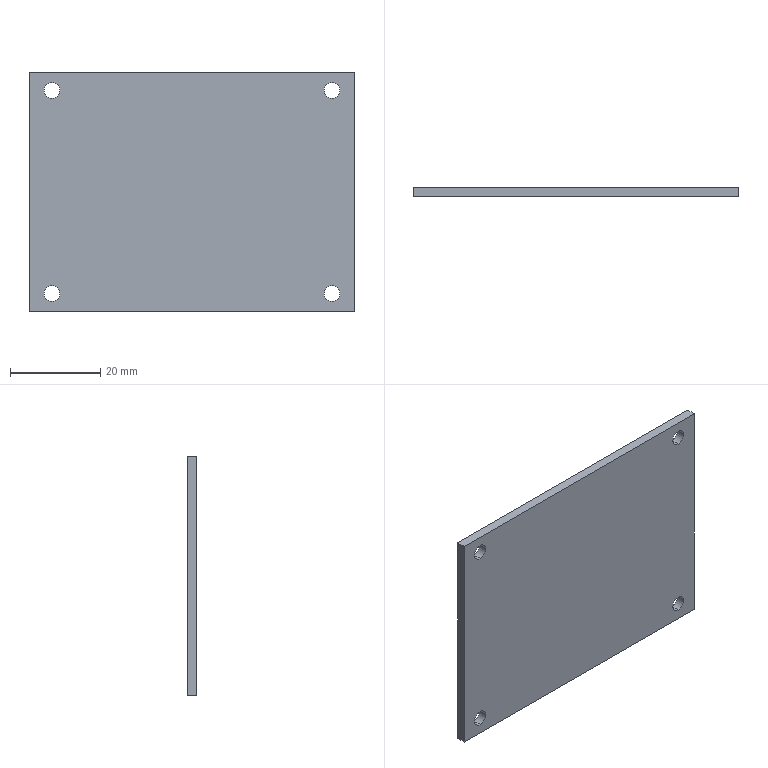Part | SolidWorks | features BaseBody 1 | 1 solid | 14 faces | box 72 x 2 x 53 mm | volume 7555 mm3 | cylinder 8 | plane 6 | commonest cylinder face diameters 3.5 x8
STEP:
#1=CARTESIAN_POINT('',(-31.,2.,24.25));
#2=VERTEX_POINT('',#1);
#3=CARTESIAN_POINT('',(-31.,0.,24.25));
#4=VERTEX_POINT('',#3);
#5=CARTESIAN_POINT('',(-31.,2.,24.25));
#6=DIRECTION('',(0.,-1.,0.));
#7=VECTOR('',#6,1000.);
#8=LINE('',#5,#7);
#9=EDGE_CURVE('',#2,#4,#8,.T.);
#10=ORIENTED_EDGE('',*,*,#9,.F.);
#11=CARTESIAN_POINT('',(-31.,2.,20.75));
#12=VERTEX_POINT('',#11);
#13=CARTESIAN_POINT('',(-31.,2.,22.5));
#14=DIRECTION('',(0.,1.,0.));
#15=DIRECTION('',(0.,0.,-1.));
#16=AXIS2_PLACEMENT_3D('',#13,#14,#15);
#17=CIRCLE('',#16,1.75);
#18=EDGE_CURVE('',#2,#12,#17,.T.);
#19=ORIENTED_EDGE('',*,*,#18,.T.);
#20=CARTESIAN_POINT('',(-31.,0.,20.75));
#21=VERTEX_POINT('',#20);
#22=CARTESIAN_POINT('',(-31.,2.,20.75));
#23=DIRECTION('',(0.,-1.,0.));
#24=VECTOR('',#23,1000.);
#25=LINE('',#22,#24);
#26=EDGE_CURVE('',#12,#21,#25,.T.);
#27=ORIENTED_EDGE('',*,*,#26,.T.);
#28=CARTESIAN_POINT('',(-31.,0.,22.5));
#29=DIRECTION('',(0.,1.,0.));
#30=DIRECTION('',(0.,0.,-1.));
#31=AXIS2_PLACEMENT_3D('',#28,#29,#30);
#32=CIRCLE('',#31,1.75);
#33=EDGE_CURVE('',#4,#21,#32,.T.);
#34=ORIENTED_EDGE('',*,*,#33,.F.);
#35=EDGE_LOOP('',(#10,#19,#27,#34));
#36=FACE_OUTER_BOUND('',#35,.T.);
#37=CARTESIAN_POINT('',(-31.,2.,22.5));
#38=DIRECTION('',(0.,-1.,0.));
#39=DIRECTION('',(0.,0.,-1.));
#40=AXIS2_PLACEMENT_3D('',#37,#38,#39);
#41=CYLINDRICAL_SURFACE('',#40,1.75);
#42=ADVANCED_FACE('',(#36),#41,.F.);
#43=CARTESIAN_POINT('',(31.,2.,24.25));
#44=VERTEX_POINT('',#43);
#45=CARTESIAN_POINT('',(31.,0.,24.25));
#46=VERTEX_POINT('',#45);
#47=CARTESIAN_POINT('',(31.,2.,24.25));
#48=DIRECTION('',(0.,-1.,0.));
#49=VECTOR('',#48,1000.);
#50=LINE('',#47,#49);
#51=EDGE_CURVE('',#44,#46,#50,.T.);
#52=ORIENTED_EDGE('',*,*,#51,.F.);
#53=CARTESIAN_POINT('',(31.,2.,20.75));
#54=VERTEX_POINT('',#53);
#55=CARTESIAN_POINT('',(31.,2.,22.5));
#56=DIRECTION('',(0.,1.,0.));
#57=DIRECTION('',(0.,0.,1.));
#58=AXIS2_PLACEMENT_3D('',#55,#56,#57);
#59=CIRCLE('',#58,1.75);
#60=EDGE_CURVE('',#44,#54,#59,.T.);
#61=ORIENTED_EDGE('',*,*,#60,.T.);
#62=CARTESIAN_POINT('',(31.,0.,20.75));
#63=VERTEX_POINT('',#62);
#64=CARTESIAN_POINT('',(31.,2.,20.75));
#65=DIRECTION('',(0.,-1.,0.));
#66=VECTOR('',#65,1000.);
#67=LINE('',#64,#66);
#68=EDGE_CURVE('',#54,#63,#67,.T.);
#69=ORIENTED_EDGE('',*,*,#68,.T.);
#70=CARTESIAN_POINT('',(31.,0.,22.5));
#71=DIRECTION('',(0.,1.,0.));
#72=DIRECTION('',(0.,0.,1.));
#73=AXIS2_PLACEMENT_3D('',#70,#71,#72);
#74=CIRCLE('',#73,1.75);
#75=EDGE_CURVE('',#46,#63,#74,.T.);
#76=ORIENTED_EDGE('',*,*,#75,.F.);
#77=EDGE_LOOP('',(#52,#61,#69,#76));
#78=FACE_OUTER_BOUND('',#77,.T.);
#79=CARTESIAN_POINT('',(31.,2.,22.5));
#80=DIRECTION('',(0.,-1.,0.));
#81=DIRECTION('',(0.,0.,-1.));
#82=AXIS2_PLACEMENT_3D('',#79,#80,#81);
#83=CYLINDRICAL_SURFACE('',#82,1.75);
#84=ADVANCED_FACE('',(#78),#83,.F.);
#85=CARTESIAN_POINT('',(31.,2.,-20.75));
#86=VERTEX_POINT('',#85);
#87=CARTESIAN_POINT('',(31.,0.,-20.75));
#88=VERTEX_POINT('',#87);
#89=CARTESIAN_POINT('',(31.,2.,-20.75));
#90=DIRECTION('',(0.,-1.,0.));
#91=VECTOR('',#90,1000.);
#92=LINE('',#89,#91);
#93=EDGE_CURVE('',#86,#88,#92,.T.);
#94=ORIENTED_EDGE('',*,*,#93,.F.);
#95=CARTESIAN_POINT('',(31.,2.,-24.25));
#96=VERTEX_POINT('',#95);
#97=CARTESIAN_POINT('',(31.,2.,-22.5));
#98=DIRECTION('',(0.,1.,0.));
#99=DIRECTION('',(0.,0.,-1.));
#100=AXIS2_PLACEMENT_3D('',#97,#98,#99);
#101=CIRCLE('',#100,1.75);
#102=EDGE_CURVE('',#86,#96,#101,.T.);
#103=ORIENTED_EDGE('',*,*,#102,.T.);
#104=CARTESIAN_POINT('',(31.,0.,-24.25));
#105=VERTEX_POINT('',#104);
#106=CARTESIAN_POINT('',(31.,2.,-24.25));
#107=DIRECTION('',(0.,-1.,0.));
#108=VECTOR('',#107,1000.);
#109=LINE('',#106,#108);
#110=EDGE_CURVE('',#96,#105,#109,.T.);
#111=ORIENTED_EDGE('',*,*,#110,.T.);
#112=CARTESIAN_POINT('',(31.,0.,-22.5));
#113=DIRECTION('',(0.,1.,0.));
#114=DIRECTION('',(0.,0.,-1.));
#115=AXIS2_PLACEMENT_3D('',#112,#113,#114);
#116=CIRCLE('',#115,1.75);
#117=EDGE_CURVE('',#88,#105,#116,.T.);
#118=ORIENTED_EDGE('',*,*,#117,.F.);
#119=EDGE_LOOP('',(#94,#103,#111,#118));
#120=FACE_OUTER_BOUND('',#119,.T.);
#121=CARTESIAN_POINT('',(31.,2.,-22.5));
#122=DIRECTION('',(0.,-1.,0.));
#123=DIRECTION('',(0.,0.,-1.));
#124=AXIS2_PLACEMENT_3D('',#121,#122,#123);
#125=CYLINDRICAL_SURFACE('',#124,1.75);
#126=ADVANCED_FACE('',(#120),#125,.F.);
#127=CARTESIAN_POINT('',(-31.,2.,-20.75));
#128=VERTEX_POINT('',#127);
#129=CARTESIAN_POINT('',(-31.,0.,-20.75));
#130=VERTEX_POINT('',#129);
#131=CARTESIAN_POINT('',(-31.,2.,-20.75));
#132=DIRECTION('',(0.,-1.,0.));
#133=VECTOR('',#132,1000.);
#134=LINE('',#131,#133);
#135=EDGE_CURVE('',#128,#130,#134,.T.);
#136=ORIENTED_EDGE('',*,*,#135,.F.);
#137=CARTESIAN_POINT('',(-31.,2.,-24.25));
#138=VERTEX_POINT('',#137);
#139=CARTESIAN_POINT('',(-31.,2.,-22.5));
#140=DIRECTION('',(0.,1.,0.));
#141=DIRECTION('',(0.,0.,1.));
#142=AXIS2_PLACEMENT_3D('',#139,#140,#141);
#143=CIRCLE('',#142,1.75);
#144=EDGE_CURVE('',#128,#138,#143,.T.);
#145=ORIENTED_EDGE('',*,*,#144,.T.);
#146=CARTESIAN_POINT('',(-31.,0.,-24.25));
#147=VERTEX_POINT('',#146);
#148=CARTESIAN_POINT('',(-31.,2.,-24.25));
#149=DIRECTION('',(0.,-1.,0.));
#150=VECTOR('',#149,1000.);
#151=LINE('',#148,#150);
#152=EDGE_CURVE('',#138,#147,#151,.T.);
#153=ORIENTED_EDGE('',*,*,#152,.T.);
#154=CARTESIAN_POINT('',(-31.,0.,-22.5));
#155=DIRECTION('',(0.,1.,0.));
#156=DIRECTION('',(0.,0.,1.));
#157=AXIS2_PLACEMENT_3D('',#154,#155,#156);
#158=CIRCLE('',#157,1.75);
#159=EDGE_CURVE('',#130,#147,#158,.T.);
#160=ORIENTED_EDGE('',*,*,#159,.F.);
#161=EDGE_LOOP('',(#136,#145,#153,#160));
#162=FACE_OUTER_BOUND('',#161,.T.);
#163=CARTESIAN_POINT('',(-31.,2.,-22.5));
#164=DIRECTION('',(0.,-1.,0.));
#165=DIRECTION('',(0.,0.,-1.));
#166=AXIS2_PLACEMENT_3D('',#163,#164,#165);
#167=CYLINDRICAL_SURFACE('',#166,1.75);
#168=ADVANCED_FACE('',(#162),#167,.F.);
#169=CARTESIAN_POINT('',(-36.,0.,26.5));
#170=VERTEX_POINT('',#169);
#171=CARTESIAN_POINT('',(36.,0.,26.5));
#172=VERTEX_POINT('',#171);
#173=CARTESIAN_POINT('',(-36.,0.,26.5));
#174=DIRECTION('',(1.,0.,0.));
#175=VECTOR('',#174,1000.);
#176=LINE('',#173,#175);
#177=EDGE_CURVE('',#170,#172,#176,.T.);
#178=ORIENTED_EDGE('',*,*,#177,.T.);
#179=CARTESIAN_POINT('',(36.,2.,26.5));
#180=VERTEX_POINT('',#179);
#181=CARTESIAN_POINT('',(36.,2.,26.5));
#182=DIRECTION('',(0.,-1.,0.));
#183=VECTOR('',#182,1000.);
#184=LINE('',#181,#183);
#185=EDGE_CURVE('',#180,#172,#184,.T.);
#186=ORIENTED_EDGE('',*,*,#185,.F.);
#187=CARTESIAN_POINT('',(-36.,2.,26.5));
#188=VERTEX_POINT('',#187);
#189=CARTESIAN_POINT('',(-36.,2.,26.5));
#190=DIRECTION('',(1.,0.,0.));
#191=VECTOR('',#190,1000.);
#192=LINE('',#189,#191);
#193=EDGE_CURVE('',#188,#180,#192,.T.);
#194=ORIENTED_EDGE('',*,*,#193,.F.);
#195=CARTESIAN_POINT('',(-36.,2.,26.5));
#196=DIRECTION('',(0.,-1.,0.));
#197=VECTOR('',#196,1000.);
#198=LINE('',#195,#197);
#199=EDGE_CURVE('',#188,#170,#198,.T.);
#200=ORIENTED_EDGE('',*,*,#199,.T.);
#201=EDGE_LOOP('',(#178,#186,#194,#200));
#202=FACE_OUTER_BOUND('',#201,.T.);
#203=CARTESIAN_POINT('',(-36.,2.,26.5));
#204=DIRECTION('',(0.,0.,-1.));
#205=DIRECTION('',(0.,-1.,0.));
#206=AXIS2_PLACEMENT_3D('',#203,#204,#205);
#207=PLANE('',#206);
#208=ADVANCED_FACE('',(#202),#207,.F.);
#209=CARTESIAN_POINT('',(-36.,0.,-26.5));
#210=VERTEX_POINT('',#209);
#211=CARTESIAN_POINT('',(-36.,0.,-26.5));
#212=DIRECTION('',(0.,0.,1.));
#213=VECTOR('',#212,1000.);
#214=LINE('',#211,#213);
#215=EDGE_CURVE('',#210,#170,#214,.T.);
#216=ORIENTED_EDGE('',*,*,#215,.T.);
#217=ORIENTED_EDGE('',*,*,#199,.F.);
#218=CARTESIAN_POINT('',(-36.,2.,-26.5));
#219=VERTEX_POINT('',#218);
#220=CARTESIAN_POINT('',(-36.,2.,-26.5));
#221=DIRECTION('',(0.,0.,1.));
#222=VECTOR('',#221,1000.);
#223=LINE('',#220,#222);
#224=EDGE_CURVE('',#219,#188,#223,.T.);
#225=ORIENTED_EDGE('',*,*,#224,.F.);
#226=CARTESIAN_POINT('',(-36.,2.,-26.5));
#227=DIRECTION('',(0.,-1.,0.));
#228=VECTOR('',#227,1000.);
#229=LINE('',#226,#228);
#230=EDGE_CURVE('',#219,#210,#229,.T.);
#231=ORIENTED_EDGE('',*,*,#230,.T.);
#232=EDGE_LOOP('',(#216,#217,#225,#231));
#233=FACE_OUTER_BOUND('',#232,.T.);
#234=CARTESIAN_POINT('',(-36.,2.,-26.5));
#235=DIRECTION('',(1.,0.,0.));
#236=DIRECTION('',(0.,1.,0.));
#237=AXIS2_PLACEMENT_3D('',#234,#235,#236);
#238=PLANE('',#237);
#239=ADVANCED_FACE('',(#233),#238,.F.);
#240=CARTESIAN_POINT('',(36.,0.,-26.5));
#241=VERTEX_POINT('',#240);
#242=CARTESIAN_POINT('',(-36.,0.,-26.5));
#243=DIRECTION('',(-1.,0.,0.));
#244=VECTOR('',#243,1000.);
#245=LINE('',#242,#244);
#246=EDGE_CURVE('',#241,#210,#245,.T.);
#247=ORIENTED_EDGE('',*,*,#246,.T.);
#248=ORIENTED_EDGE('',*,*,#230,.F.);
#249=CARTESIAN_POINT('',(36.,2.,-26.5));
#250=VERTEX_POINT('',#249);
#251=CARTESIAN_POINT('',(-36.,2.,-26.5));
#252=DIRECTION('',(-1.,0.,0.));
#253=VECTOR('',#252,1000.);
#254=LINE('',#251,#253);
#255=EDGE_CURVE('',#250,#219,#254,.T.);
#256=ORIENTED_EDGE('',*,*,#255,.F.);
#257=CARTESIAN_POINT('',(36.,2.,-26.5));
#258=DIRECTION('',(0.,-1.,0.));
#259=VECTOR('',#258,1000.);
#260=LINE('',#257,#259);
#261=EDGE_CURVE('',#250,#241,#260,.T.);
#262=ORIENTED_EDGE('',*,*,#261,.T.);
#263=EDGE_LOOP('',(#247,#248,#256,#262));
#264=FACE_OUTER_BOUND('',#263,.T.);
#265=CARTESIAN_POINT('',(-36.,2.,-26.5));
#266=DIRECTION('',(0.,0.,1.));
#267=DIRECTION('',(1.,0.,0.));
#268=AXIS2_PLACEMENT_3D('',#265,#266,#267);
#269=PLANE('',#268);
#270=ADVANCED_FACE('',(#264),#269,.F.);
#271=CARTESIAN_POINT('',(36.,0.,-26.5));
#272=DIRECTION('',(0.,0.,-1.));
#273=VECTOR('',#272,1000.);
#274=LINE('',#271,#273);
#275=EDGE_CURVE('',#172,#241,#274,.T.);
#276=ORIENTED_EDGE('',*,*,#275,.T.);
#277=ORIENTED_EDGE('',*,*,#261,.F.);
#278=CARTESIAN_POINT('',(36.,2.,-26.5));
#279=DIRECTION('',(0.,0.,-1.));
#280=VECTOR('',#279,1000.);
#281=LINE('',#278,#280);
#282=EDGE_CURVE('',#180,#250,#281,.T.);
#283=ORIENTED_EDGE('',*,*,#282,.F.);
#284=ORIENTED_EDGE('',*,*,#185,.T.);
#285=EDGE_LOOP('',(#276,#277,#283,#284));
#286=FACE_OUTER_BOUND('',#285,.T.);
#287=CARTESIAN_POINT('',(36.,2.,-26.5));
#288=DIRECTION('',(-1.,0.,0.));
#289=DIRECTION('',(0.,1.,0.));
#290=AXIS2_PLACEMENT_3D('',#287,#288,#289);
#291=PLANE('',#290);
#292=ADVANCED_FACE('',(#286),#291,.F.);
#293=CARTESIAN_POINT('',(-31.,0.,22.5));
#294=DIRECTION('',(0.,1.,0.));
#295=DIRECTION('',(0.,0.,-1.));
#296=AXIS2_PLACEMENT_3D('',#293,#294,#295);
#297=CIRCLE('',#296,1.75);
#298=EDGE_CURVE('',#21,#4,#297,.T.);
#299=ORIENTED_EDGE('',*,*,#298,.T.);
#300=ORIENTED_EDGE('',*,*,#33,.T.);
#301=EDGE_LOOP('',(#299,#300));
#302=FACE_BOUND('',#301,.T.);
#303=CARTESIAN_POINT('',(31.,0.,22.5));
#304=DIRECTION('',(0.,1.,0.));
#305=DIRECTION('',(0.,0.,1.));
#306=AXIS2_PLACEMENT_3D('',#303,#304,#305);
#307=CIRCLE('',#306,1.75);
#308=EDGE_CURVE('',#63,#46,#307,.T.);
#309=ORIENTED_EDGE('',*,*,#308,.T.);
#310=ORIENTED_EDGE('',*,*,#75,.T.);
#311=EDGE_LOOP('',(#309,#310));
#312=FACE_BOUND('',#311,.T.);
#313=CARTESIAN_POINT('',(31.,0.,-22.5));
#314=DIRECTION('',(0.,1.,0.));
#315=DIRECTION('',(0.,0.,-1.));
#316=AXIS2_PLACEMENT_3D('',#313,#314,#315);
#317=CIRCLE('',#316,1.75);
#318=EDGE_CURVE('',#105,#88,#317,.T.);
#319=ORIENTED_EDGE('',*,*,#318,.T.);
#320=ORIENTED_EDGE('',*,*,#117,.T.);
#321=EDGE_LOOP('',(#319,#320));
#322=FACE_BOUND('',#321,.T.);
#323=CARTESIAN_POINT('',(-31.,0.,-22.5));
#324=DIRECTION('',(0.,1.,0.));
#325=DIRECTION('',(0.,0.,1.));
#326=AXIS2_PLACEMENT_3D('',#323,#324,#325);
#327=CIRCLE('',#326,1.75);
#328=EDGE_CURVE('',#147,#130,#327,.T.);
#329=ORIENTED_EDGE('',*,*,#328,.T.);
#330=ORIENTED_EDGE('',*,*,#159,.T.);
#331=EDGE_LOOP('',(#329,#330));
#332=FACE_BOUND('',#331,.T.);
#333=ORIENTED_EDGE('',*,*,#275,.F.);
#334=ORIENTED_EDGE('',*,*,#177,.F.);
#335=ORIENTED_EDGE('',*,*,#215,.F.);
#336=ORIENTED_EDGE('',*,*,#246,.F.);
#337=EDGE_LOOP('',(#333,#334,#335,#336));
#338=FACE_OUTER_BOUND('',#337,.T.);
#339=CARTESIAN_POINT('',(0.,0.,0.));
#340=DIRECTION('',(0.,1.,0.));
#341=DIRECTION('',(1.,0.,0.));
#342=AXIS2_PLACEMENT_3D('',#339,#340,#341);
#343=PLANE('',#342);
#344=ADVANCED_FACE('',(#302,#312,#322,#332,#338),#343,.F.);
#345=CARTESIAN_POINT('',(-31.,2.,22.5));
#346=DIRECTION('',(0.,1.,0.));
#347=DIRECTION('',(0.,0.,-1.));
#348=AXIS2_PLACEMENT_3D('',#345,#346,#347);
#349=CIRCLE('',#348,1.75);
#350=EDGE_CURVE('',#12,#2,#349,.T.);
#351=ORIENTED_EDGE('',*,*,#350,.F.);
#352=ORIENTED_EDGE('',*,*,#18,.F.);
#353=EDGE_LOOP('',(#351,#352));
#354=FACE_BOUND('',#353,.T.);
#355=CARTESIAN_POINT('',(31.,2.,-22.5));
#356=DIRECTION('',(0.,1.,0.));
#357=DIRECTION('',(0.,0.,-1.));
#358=AXIS2_PLACEMENT_3D('',#355,#356,#357);
#359=CIRCLE('',#358,1.75);
#360=EDGE_CURVE('',#96,#86,#359,.T.);
#361=ORIENTED_EDGE('',*,*,#360,.F.);
#362=ORIENTED_EDGE('',*,*,#102,.F.);
#363=EDGE_LOOP('',(#361,#362));
#364=FACE_BOUND('',#363,.T.);
#365=CARTESIAN_POINT('',(-31.,2.,-22.5));
#366=DIRECTION('',(0.,1.,0.));
#367=DIRECTION('',(0.,0.,1.));
#368=AXIS2_PLACEMENT_3D('',#365,#366,#367);
#369=CIRCLE('',#368,1.75);
#370=EDGE_CURVE('',#138,#128,#369,.T.);
#371=ORIENTED_EDGE('',*,*,#370,.F.);
#372=ORIENTED_EDGE('',*,*,#144,.F.);
#373=EDGE_LOOP('',(#371,#372));
#374=FACE_BOUND('',#373,.T.);
#375=CARTESIAN_POINT('',(31.,2.,22.5));
#376=DIRECTION('',(0.,1.,0.));
#377=DIRECTION('',(0.,0.,1.));
#378=AXIS2_PLACEMENT_3D('',#375,#376,#377);
#379=CIRCLE('',#378,1.75);
#380=EDGE_CURVE('',#54,#44,#379,.T.);
#381=ORIENTED_EDGE('',*,*,#380,.F.);
#382=ORIENTED_EDGE('',*,*,#60,.F.);
#383=EDGE_LOOP('',(#381,#382));
#384=FACE_BOUND('',#383,.T.);
#385=ORIENTED_EDGE('',*,*,#282,.T.);
#386=ORIENTED_EDGE('',*,*,#255,.T.);
#387=ORIENTED_EDGE('',*,*,#224,.T.);
#388=ORIENTED_EDGE('',*,*,#193,.T.);
#389=EDGE_LOOP('',(#385,#386,#387,#388));
#390=FACE_OUTER_BOUND('',#389,.T.);
#391=CARTESIAN_POINT('',(0.,2.,0.));
#392=DIRECTION('',(0.,1.,0.));
#393=DIRECTION('',(1.,0.,0.));
#394=AXIS2_PLACEMENT_3D('',#391,#392,#393);
#395=PLANE('',#394);
#396=ADVANCED_FACE('',(#354,#364,#374,#384,#390),#395,.T.);
#397=ORIENTED_EDGE('',*,*,#370,.T.);
#398=ORIENTED_EDGE('',*,*,#135,.T.);
#399=ORIENTED_EDGE('',*,*,#328,.F.);
#400=ORIENTED_EDGE('',*,*,#152,.F.);
#401=EDGE_LOOP('',(#397,#398,#399,#400));
#402=FACE_OUTER_BOUND('',#401,.T.);
#403=CARTESIAN_POINT('',(-31.,2.,-22.5));
#404=DIRECTION('',(0.,-1.,0.));
#405=DIRECTION('',(0.,0.,-1.));
#406=AXIS2_PLACEMENT_3D('',#403,#404,#405);
#407=CYLINDRICAL_SURFACE('',#406,1.75);
#408=ADVANCED_FACE('',(#402),#407,.F.);
#409=ORIENTED_EDGE('',*,*,#360,.T.);
#410=ORIENTED_EDGE('',*,*,#93,.T.);
#411=ORIENTED_EDGE('',*,*,#318,.F.);
#412=ORIENTED_EDGE('',*,*,#110,.F.);
#413=EDGE_LOOP('',(#409,#410,#411,#412));
#414=FACE_OUTER_BOUND('',#413,.T.);
#415=CARTESIAN_POINT('',(31.,2.,-22.5));
#416=DIRECTION('',(0.,-1.,0.));
#417=DIRECTION('',(0.,0.,-1.));
#418=AXIS2_PLACEMENT_3D('',#415,#416,#417);
#419=CYLINDRICAL_SURFACE('',#418,1.75);
#420=ADVANCED_FACE('',(#414),#419,.F.);
#421=ORIENTED_EDGE('',*,*,#380,.T.);
#422=ORIENTED_EDGE('',*,*,#51,.T.);
#423=ORIENTED_EDGE('',*,*,#308,.F.);
#424=ORIENTED_EDGE('',*,*,#68,.F.);
#425=EDGE_LOOP('',(#421,#422,#423,#424));
#426=FACE_OUTER_BOUND('',#425,.T.);
#427=CARTESIAN_POINT('',(31.,2.,22.5));
#428=DIRECTION('',(0.,-1.,0.));
#429=DIRECTION('',(0.,0.,-1.));
#430=AXIS2_PLACEMENT_3D('',#427,#428,#429);
#431=CYLINDRICAL_SURFACE('',#430,1.75);
#432=ADVANCED_FACE('',(#426),#431,.F.);
#433=ORIENTED_EDGE('',*,*,#350,.T.);
#434=ORIENTED_EDGE('',*,*,#9,.T.);
#435=ORIENTED_EDGE('',*,*,#298,.F.);
#436=ORIENTED_EDGE('',*,*,#26,.F.);
#437=EDGE_LOOP('',(#433,#434,#435,#436));
#438=FACE_OUTER_BOUND('',#437,.T.);
#439=CARTESIAN_POINT('',(-31.,2.,22.5));
#440=DIRECTION('',(0.,-1.,0.));
#441=DIRECTION('',(0.,0.,-1.));
#442=AXIS2_PLACEMENT_3D('',#439,#440,#441);
#443=CYLINDRICAL_SURFACE('',#442,1.75);
#444=ADVANCED_FACE('',(#438),#443,.F.);
#445=CLOSED_SHELL('',(#42,#84,#126,#168,#208,#239,#270,#292,#344,#396,#408,#420,#432,#444));
#446=MANIFOLD_SOLID_BREP('',#445);
#447=CARTESIAN_POINT('',(0.,0.,0.));
#448=DIRECTION('',(0.,0.,1.));
#449=DIRECTION('',(1.,0.,0.));
#450=AXIS2_PLACEMENT_3D('',#447,#448,#449);
#451=(LENGTH_UNIT()NAMED_UNIT(*)SI_UNIT(.MILLI.,.METRE.));
#452=UNCERTAINTY_MEASURE_WITH_UNIT(LENGTH_MEASURE(0.00001),#451,'','');
#453=(NAMED_UNIT(*)PLANE_ANGLE_UNIT()SI_UNIT($,.RADIAN.));
#454=(NAMED_UNIT(*)SI_UNIT($,.STERADIAN.)SOLID_ANGLE_UNIT());
#455=(GEOMETRIC_REPRESENTATION_CONTEXT(3)GLOBAL_UNCERTAINTY_ASSIGNED_CONTEXT((#452))GLOBAL_UNIT_ASSIGNED_CONTEXT((#451,#453,#454))REPRESENTATION_CONTEXT('',''));
#456=ADVANCED_BREP_SHAPE_REPRESENTATION('',(#446,#450),#455);